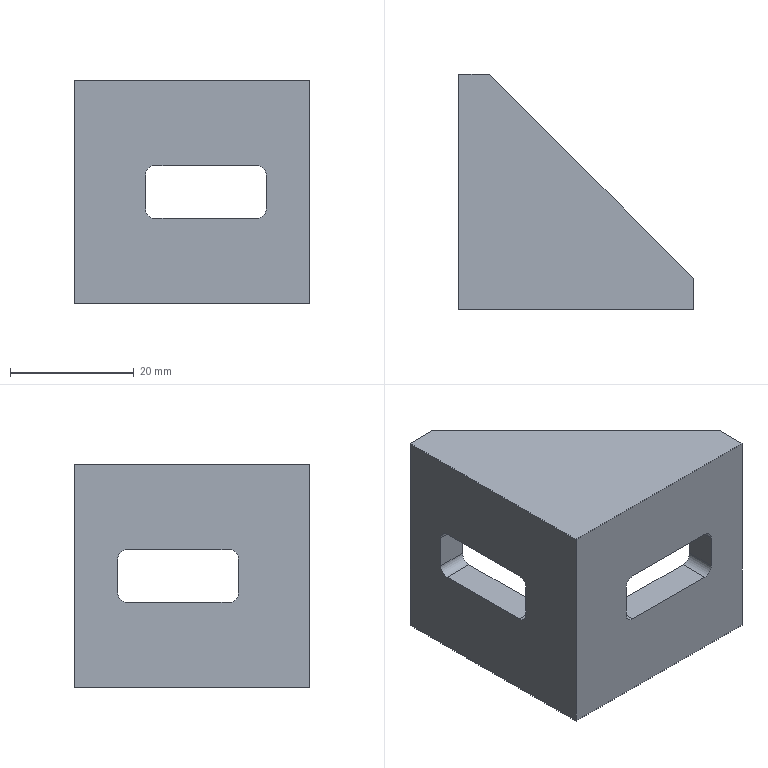Part | STEP file | Die-cast aluminium connector, 40 series, 40mm face, standard type | 1 solid | 28 faces | box 38 x 38 x 36 mm | volume 14409 mm3 | plane 20 | cylinder 8 | commonest cylinder face diameters 3 x8